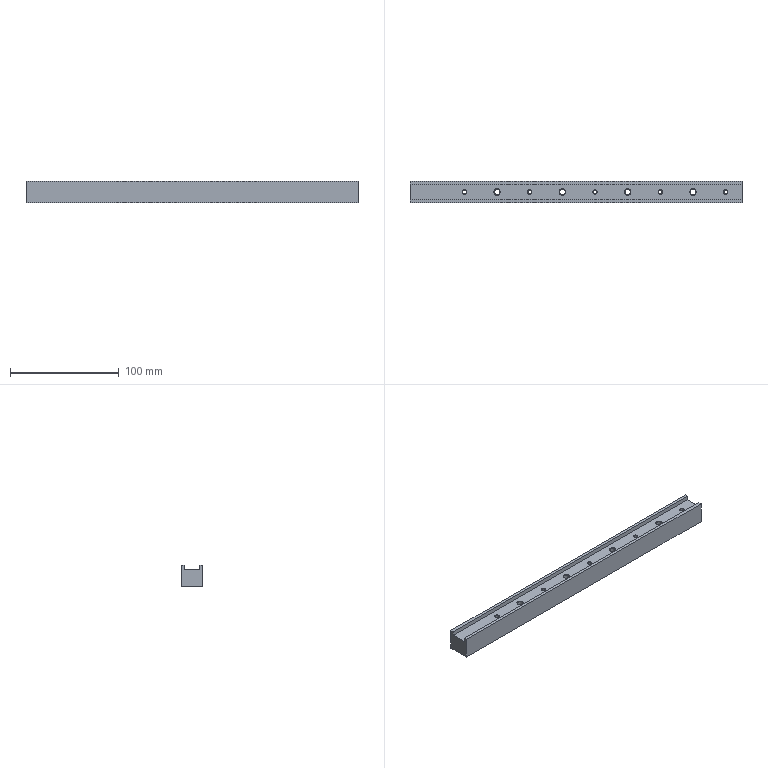Part | STEP file | Tube feed_id866_x_t | 1 solid | 37 faces | box 305 x 20 x 20 mm | volume 102341 mm3 | cone 18 | plane 10 | cylinder 9 | commonest cylinder face diameters 3.3 x5 5 x4